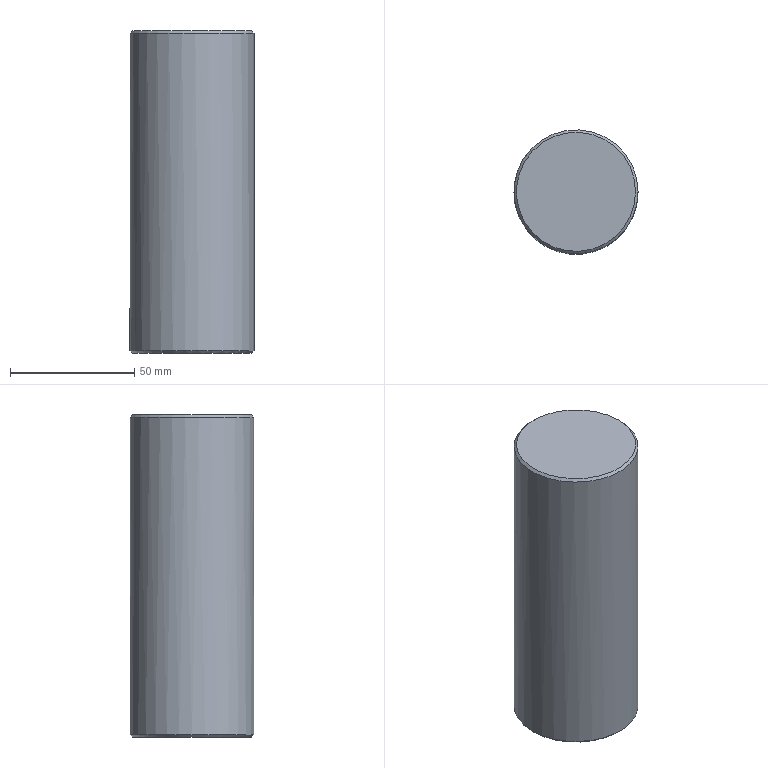Part | STEP file | SL2-MOLD_id90_xmt_txt | 1 solid | 8 faces | box 50 x 50 x 130 mm | volume 253722 mm3 | plane 3 | cone 3 | cylinder 2 | commonest cylinder face diameters 12 x1 50 x1
STEP:
#1=CARTESIAN_POINT('',(24.,285.,-114.));
#2=VERTEX_POINT('',#1);
#3=CARTESIAN_POINT('',(0.,285.,-114.));
#4=DIRECTION('',(0.,0.,1.));
#5=DIRECTION('',(1.,0.,0.));
#6=AXIS2_PLACEMENT_3D('',#3,#4,#5);
#7=CIRCLE('',#6,24.);
#8=EDGE_CURVE('',#2,#2,#7,.T.);
#9=ORIENTED_EDGE('',*,*,#8,.T.);
#10=EDGE_LOOP('',(#9));
#11=FACE_OUTER_BOUND('',#10,.T.);
#12=CARTESIAN_POINT('',(0.,285.,-114.));
#13=DIRECTION('',(0.,0.,1.));
#14=DIRECTION('',(1.,0.,0.));
#15=AXIS2_PLACEMENT_3D('',#12,#13,#14);
#16=PLANE('',#15);
#17=ADVANCED_FACE('',(#11),#16,.T.);
#18=CARTESIAN_POINT('',(-7.,285.,-244.));
#19=VERTEX_POINT('',#18);
#20=CARTESIAN_POINT('',(0.,285.,-244.));
#21=DIRECTION('',(0.,0.,1.));
#22=DIRECTION('',(-1.,0.,0.));
#23=AXIS2_PLACEMENT_3D('',#20,#21,#22);
#24=CIRCLE('',#23,7.);
#25=EDGE_CURVE('',#19,#19,#24,.T.);
#26=ORIENTED_EDGE('',*,*,#25,.T.);
#27=EDGE_LOOP('',(#26));
#28=FACE_BOUND('',#27,.T.);
#29=CARTESIAN_POINT('',(-24.,285.,-244.));
#30=VERTEX_POINT('',#29);
#31=CARTESIAN_POINT('',(0.,285.,-244.));
#32=DIRECTION('',(0.,0.,-1.));
#33=DIRECTION('',(-1.,0.,0.));
#34=AXIS2_PLACEMENT_3D('',#31,#32,#33);
#35=CIRCLE('',#34,24.);
#36=EDGE_CURVE('',#30,#30,#35,.T.);
#37=ORIENTED_EDGE('',*,*,#36,.T.);
#38=EDGE_LOOP('',(#37));
#39=FACE_BOUND('',#38,.T.);
#40=CARTESIAN_POINT('',(0.,285.,-244.));
#41=DIRECTION('',(0.,0.,-1.));
#42=DIRECTION('',(-1.,0.,0.));
#43=AXIS2_PLACEMENT_3D('',#40,#41,#42);
#44=PLANE('',#43);
#45=ADVANCED_FACE('',(#28,#39),#44,.T.);
#46=CARTESIAN_POINT('',(25.,285.,-115.));
#47=VERTEX_POINT('',#46);
#48=CARTESIAN_POINT('',(0.,285.,-115.));
#49=DIRECTION('',(0.,0.,-1.));
#50=DIRECTION('',(1.,0.,0.));
#51=AXIS2_PLACEMENT_3D('',#48,#49,#50);
#52=CIRCLE('',#51,25.);
#53=EDGE_CURVE('',#47,#47,#52,.T.);
#54=ORIENTED_EDGE('',*,*,#53,.T.);
#55=EDGE_LOOP('',(#54));
#56=FACE_BOUND('',#55,.T.);
#57=CARTESIAN_POINT('',(-25.,285.,-243.));
#58=VERTEX_POINT('',#57);
#59=CARTESIAN_POINT('',(0.,285.,-243.));
#60=DIRECTION('',(0.,0.,1.));
#61=DIRECTION('',(-1.,0.,0.));
#62=AXIS2_PLACEMENT_3D('',#59,#60,#61);
#63=CIRCLE('',#62,25.);
#64=EDGE_CURVE('',#58,#58,#63,.T.);
#65=ORIENTED_EDGE('',*,*,#64,.T.);
#66=EDGE_LOOP('',(#65));
#67=FACE_BOUND('',#66,.T.);
#68=CARTESIAN_POINT('',(0.,285.,-244.));
#69=DIRECTION('',(0.,0.,1.));
#70=DIRECTION('',(1.,0.,0.));
#71=AXIS2_PLACEMENT_3D('',#68,#69,#70);
#72=CYLINDRICAL_SURFACE('',#71,25.);
#73=ADVANCED_FACE('',(#56,#67),#72,.T.);
#74=CARTESIAN_POINT('',(6.,285.,-232.));
#75=VERTEX_POINT('',#74);
#76=CARTESIAN_POINT('',(0.,285.,-232.));
#77=DIRECTION('',(0.,0.,-1.));
#78=DIRECTION('',(1.,0.,0.));
#79=AXIS2_PLACEMENT_3D('',#76,#77,#78);
#80=CIRCLE('',#79,6.);
#81=EDGE_CURVE('',#75,#75,#80,.T.);
#82=ORIENTED_EDGE('',*,*,#81,.T.);
#83=EDGE_LOOP('',(#82));
#84=FACE_OUTER_BOUND('',#83,.T.);
#85=CARTESIAN_POINT('',(0.,285.,-232.));
#86=DIRECTION('',(0.,0.,1.));
#87=DIRECTION('',(-1.,0.,0.));
#88=AXIS2_PLACEMENT_3D('',#85,#86,#87);
#89=PLANE('',#88);
#90=ADVANCED_FACE('',(#84),#89,.F.);
#91=CARTESIAN_POINT('',(-6.,285.,-243.));
#92=VERTEX_POINT('',#91);
#93=CARTESIAN_POINT('',(0.,285.,-243.));
#94=DIRECTION('',(0.,0.,-1.));
#95=DIRECTION('',(-1.,0.,0.));
#96=AXIS2_PLACEMENT_3D('',#93,#94,#95);
#97=CIRCLE('',#96,6.);
#98=EDGE_CURVE('',#92,#92,#97,.T.);
#99=ORIENTED_EDGE('',*,*,#98,.T.);
#100=EDGE_LOOP('',(#99));
#101=FACE_BOUND('',#100,.T.);
#102=ORIENTED_EDGE('',*,*,#81,.F.);
#103=EDGE_LOOP('',(#102));
#104=FACE_BOUND('',#103,.T.);
#105=CARTESIAN_POINT('',(0.,285.,79.5));
#106=DIRECTION('',(0.,0.,-1.));
#107=DIRECTION('',(-1.,0.,0.));
#108=AXIS2_PLACEMENT_3D('',#105,#106,#107);
#109=CYLINDRICAL_SURFACE('',#108,6.);
#110=ADVANCED_FACE('',(#101,#104),#109,.F.);
#111=ORIENTED_EDGE('',*,*,#8,.F.);
#112=EDGE_LOOP('',(#111));
#113=FACE_BOUND('',#112,.T.);
#114=ORIENTED_EDGE('',*,*,#53,.F.);
#115=EDGE_LOOP('',(#114));
#116=FACE_BOUND('',#115,.T.);
#117=CARTESIAN_POINT('',(0.,285.,-115.));
#118=DIRECTION('',(0.,0.,-1.));
#119=DIRECTION('',(-1.,0.,0.));
#120=AXIS2_PLACEMENT_3D('',#117,#118,#119);
#121=CONICAL_SURFACE('',#120,25.,45.);
#122=ADVANCED_FACE('',(#113,#116),#121,.T.);
#123=ORIENTED_EDGE('',*,*,#98,.F.);
#124=EDGE_LOOP('',(#123));
#125=FACE_BOUND('',#124,.T.);
#126=ORIENTED_EDGE('',*,*,#25,.F.);
#127=EDGE_LOOP('',(#126));
#128=FACE_BOUND('',#127,.T.);
#129=CARTESIAN_POINT('',(0.,285.,-244.));
#130=DIRECTION('',(0.,0.,-1.));
#131=DIRECTION('',(-1.,0.,0.));
#132=AXIS2_PLACEMENT_3D('',#129,#130,#131);
#133=CONICAL_SURFACE('',#132,7.,45.);
#134=ADVANCED_FACE('',(#125,#128),#133,.F.);
#135=ORIENTED_EDGE('',*,*,#36,.F.);
#136=EDGE_LOOP('',(#135));
#137=FACE_BOUND('',#136,.T.);
#138=ORIENTED_EDGE('',*,*,#64,.F.);
#139=EDGE_LOOP('',(#138));
#140=FACE_BOUND('',#139,.T.);
#141=CARTESIAN_POINT('',(0.,285.,-243.));
#142=DIRECTION('',(0.,0.,1.));
#143=DIRECTION('',(1.,0.,0.));
#144=AXIS2_PLACEMENT_3D('',#141,#142,#143);
#145=CONICAL_SURFACE('',#144,25.,45.);
#146=ADVANCED_FACE('',(#137,#140),#145,.T.);
#147=CLOSED_SHELL('',(#17,#45,#73,#90,#110,#122,#134,#146));
#148=MANIFOLD_SOLID_BREP('',#147);
#149=(LENGTH_UNIT()NAMED_UNIT(*)SI_UNIT(.MILLI.,.METRE.));
#150=UNCERTAINTY_MEASURE_WITH_UNIT(LENGTH_MEASURE(0.00002),#149,'','');
#151=(NAMED_UNIT(*)PLANE_ANGLE_UNIT()SI_UNIT($,.RADIAN.));
#152=PLANE_ANGLE_MEASURE_WITH_UNIT(PLANE_ANGLE_MEASURE(0.01745),#151);
#153=DIMENSIONAL_EXPONENTS(0.,0.,0.,0.,0.,0.,0.);
#154=(CONVERSION_BASED_UNIT('DEGREE',#152)NAMED_UNIT(#153)PLANE_ANGLE_UNIT());
#155=(NAMED_UNIT(*)SI_UNIT($,.STERADIAN.)SOLID_ANGLE_UNIT());
#156=(GEOMETRIC_REPRESENTATION_CONTEXT(3)GLOBAL_UNCERTAINTY_ASSIGNED_CONTEXT((#150))GLOBAL_UNIT_ASSIGNED_CONTEXT((#149,#154,#155))REPRESENTATION_CONTEXT('',''));
#157=ADVANCED_BREP_SHAPE_REPRESENTATION('',(#148),#156);